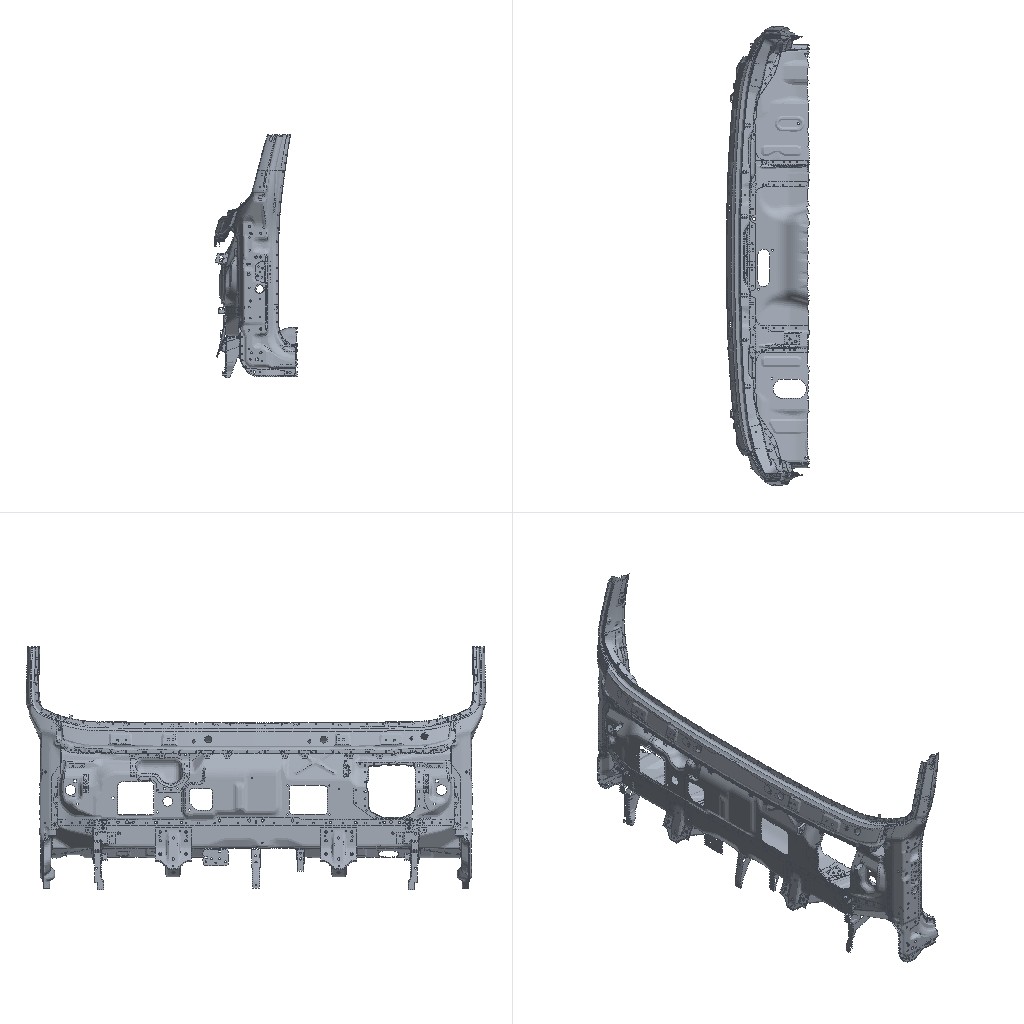Simulation study | nastran
Set-up summary:
category,name,step,type,value,unit,region
solver,nx_nastran
units,not stated in the deck,,not stated
analysis,deck,,static,static
analysis,solution,,SOL,101
load_step,SUBCASE 2,2,SUBCASE,SPC=11 LOAD=2
load_step,SUBCASE 3,3,SUBCASE,SPC=11 LOAD=3
load_step,SUBCASE 4,4,SUBCASE,SPC=11 LOAD=4
load_step,SUBCASE 5,5,SUBCASE,SPC=11 LOAD=5
load_step,SUBCASE 6,6,SUBCASE,SPC=11 LOAD=6
load_step,SUBCASE 7,7,SUBCASE,SPC=11 LOAD=7
load_step,SUBCASE 8,8,SUBCASE,SPC=11 LOAD=8
load_step,SUBCASE 9,9,SUBCASE,SPC=11 LOAD=9
load_step,SUBCASE 10,10,SUBCASE,SPC=11 LOAD=10
load_step,requested,,,9
mesh,nodes,,,77720
mesh,elements,,,69950
element_type,CHEXA,,unverified,613
element_type,CONM2,,mass,1
element_type,CQUAD4,,shell,64961
element_type,CTRIA3,,shell,4988
load,load commands in deck,,count,9
bc,support commands in deck,,count,1019
check,setup vs results,,match,"every grid point's frame and coordinates and every element id; grid points of CHEXA, CQUAD4, CTRIA3 elements"
Nastran input file, long lists of numbers shortened:
$$------------------------------------------------------------------------------$
$$                                                                              $
$$ NASTRAN Input Deck Generated by HyperMesh Version  : 9.0b121                 $
$$ Generated using HyperMesh-Nastran Template Version : 9.0b121
$$                                                                              $
$$   Template:  general                                                         $
$$                                                                              $
$$------------------------------------------------------------------------------$
$$------------------------------------------------------------------------------$
$$                      Executive Control Cards                                 $
$$------------------------------------------------------------------------------$
SOL 101
CEND
$$------------------------------------------------------------------------------$
$$                      Case Control Cards                                      $
$$------------------------------------------------------------------------------$
  DISPLACEMENT = ALL
$
$HMNAME LOADSTEP               2"Rx"
SUBCASE       2
  LABEL=   Rx
  SPC =       11
  LOAD =        2
$
$HMNAME LOADSTEP               3"Ry"
SUBCASE       3
  LABEL=   Ry
  SPC =       11
  LOAD =        3
$
$HMNAME LOADSTEP               4"Rz"
SUBCASE       4
  LABEL=   Rz
  SPC =       11
  LOAD =        4
$
$HMNAME LOADSTEP               5"Mx"
SUBCASE       5
  LABEL=   Mx
  SPC =       11
  LOAD =        5
$
$HMNAME LOADSTEP               6"My"
SUBCASE       6
  LABEL=   My
  SPC =       11
  LOAD =        6
$
$HMNAME LOADSTEP               7"Mz"
SUBCASE       7
  LABEL=   Mz
  SPC =       11
  LOAD =        7
$
$HMNAME LOADSTEP               8"Lx"
SUBCASE       8
  LABEL=   Lx
  SPC =       11
  LOAD =        8
$
$HMNAME LOADSTEP               9"Ly"
SUBCASE       9
  LABEL=   Ly
  SPC =       11
  LOAD =        9
$
$HMNAME LOADSTEP              10"Lz"
SUBCASE      10
  LABEL=   Lz
  SPC =       11
  LOAD =       10
$$------------------------------------------------------------------------------$
$$                      Bulk Data Cards                                         $
$$------------------------------------------------------------------------------$
BEGIN BULK
PARAM,POST,-1
$$
$$  GRID Data
$$
GRID         150        -903.017-1033.041012.706
GRID         536        -985.883-1013.11735.4542
$ (77718 more lines like these left out)
$$
$$  SPOINT Data
$$
$
$  CONM2 Elements
$
CONM2    103453984121617       00.00412 0.0     0.0     0.0
$
$HMMOVE 84022690
$        1034539
$
$$
$$------------------------------------------------------------------------------$
$$             Group Definitions                                                $
$$------------------------------------------------------------------------------$
$
$ RBE2 Elements - Single dependent node
$
RBE2      346590 3663307  123456 3657894
RBE2      346592 3663309  123456 3657892
$ (23 more lines like these left out)
$
$HMMOVE 57005014
$         346590  346592THRU      346597  346600THRU      346603  346605THRU
$         346608  346610THRU      346612  346614THRU      346620
$
$$
$$ RBE2 Elements - Multiple dependent nodes
$$
RBE2      346588 3663313  123456 3658184 3658185
RBE2      346589 3663312  123456 3657889 3658186
$ (98 more lines like these left out)
$
$HMMOVE 57005014
$         346588THRU      346589  346591  346598THRU      346599  346604  346609
$         346613  346621  346623THRU      346634 1034541THRU     1034542 1034540
$
$
$  RBE3 Elements
$
RBE3      326301         3755368  1234560.294793     123 37252000.075522+
+            123 37251970.128418     123 37251930.501266     123 3725196
RBE3      326302         3755369  1234560.049321     123 37252000.318302+
+            123 37251970.547536     123 37251930.084841     123 3725196
$ (9804 more lines like these left out)
$
$HMMOVE 57005012
$         326301THRU      326304  326306THRU      326313  326315THRU      326322
$         326324THRU      326331  326333THRU      326336  326427THRU      326430
$ (227 more lines like these left out)
CTRIA3    143987       2   55842   55843   55841
CTRIA3    144058       2   55842   55841   55996
$ (4986 more lines like these left out)
$
$HMMOVE       16
$         143987  144058  170026  170031  170036THRU      170037  170041  170048
$         170053  170057THRU      170058  189522  189524  198834THRU      198835
$ (604 more lines like these left out)
CQUAD4    170025       2   86431   86432   86426   86427
CQUAD4    170027       2   86442   86467   86451   86441
$ (64959 more lines like these left out)
$
$HMMOVE       16
$         170025  170027THRU      170030  170032THRU      170035  170038THRU
$         170040  170042THRU      170047  170049THRU      170052  170054THRU
$ (1536 more lines like these left out)
CHEXA     326305      10 3755368 3755369 3755370 3755371 3755372 3755373+
+        3755374 3755375
CHEXA     326314      10 3755377 3755380 3755379 3755378 3755381 3755384+
+        3755383 3755382
$ (1222 more lines like these left out)
$
$HMMOVE 57005011
$         326305  326314  326323  326332  326431  326440  326449  326458  326467
$         326476  326629  326638  326647  326656  326665  326674  326683  326692
$ (251 more lines like these left out)
PSHELL         1       10.8            1               1
$
$HMNAME PROP                   2"120" 4
$HWCOLOR PROP                  2       3
PSHELL         2       11.2            1               1
$
$HMNAME PROP                   3"180" 4
$HWCOLOR PROP                  3       3
PSHELL         3       11.8            1               1
$
$HMNAME PROP                   4"100" 4
$HWCOLOR PROP                  4       3
PSHELL         4       11.0            1               1
$
$HMNAME PROP                   5"150" 4
$HWCOLOR PROP                  5       3
PSHELL         5       11.5            1               1
$
$HMNAME PROP                   6"250" 4
$HWCOLOR PROP                  6       3
PSHELL         6       12.5            1               1
$
$HMNAME PROP                   7"200" 4
$HWCOLOR PROP                  7       3
PSHELL         7       12.0            1               1
$$
$$  PSOLID Data
$
$HMNAME PROP                  10"spot" 5
$HWCOLOR PROP                 10       3
PSOLID        10       1
$$
$$------------------------------------------------------------------------------$
$$                      Material Definition Cards                               $
$$------------------------------------------------------------------------------$
$$--------------------------------------------------------------
$$ HYPERMESH TAGS
$$--------------------------------------------------------------
$$BEGIN TAGS
$$END TAGS
$$
$$  MAT1 Data
$
$HMNAME MAT                    1"steel" "MAT1"
$HWCOLOR MAT                   1       3
MAT1           1210000.0        0.3     1.60E-08
$$
$$
$$
$$------------------------------------------------------------------------------$
$ (61 more lines like these left out)
SPC           11 3750681  1234560.0
SPC           11 3750682  1234560.0
SPC           11 3751236  1234560.0
SPC           11 3751237  1234560.0
$ (1015 more lines like these left out)
$$
$$  FORCE Data
$$
FORCE          284121625       01.0     100.0   0.0     0.0
FORCE          384121625       01.0     0.0     100.0   0.0
FORCE          484121625       01.0     0.0     0.0     100.0
FORCE          584121629       01.0     100.0   0.0     0.0
FORCE          684121629       01.0     0.0     100.0   0.0
FORCE          784121629       01.0     0.0     0.0     100.0
FORCE          884121633       01.0     100.0   0.0     0.0
FORCE          984121633       01.0     0.0     100.0   0.0
FORCE         1084121633       01.0     0.0     0.0     100.0
$HMASSEM 5400100       7 sidebody_L
$HMASSEM_IDS    540010105400303054003020540011105400112054003010
$HMASSEM 5400200       6 sidebody_R
$HMASSEM_IDS    540021105400212054004010540040205400403054002010
$HMASSEM      28       4 5300010
$HMASSEM_IDS          16      17      18      19      20      21      22      24
$HMASSEM_IDS          25      26
$HMASSEM       1       3 REAR_FLOOR
$HMASSEM_IDS    5100301051001110510052115100451051004210510048115100431151004610
$HMASSEM_IDS    5100411051002110510044105100601051009710510062115100471051004511
$HMASSEM_IDS    5100561351005410510064105100561051005611510056125100431051005311
$HMASSEM_IDS    510050105100341051009711
$
ENDDATA
Results summary:
result,analysis,,,static
result,last_loadstep,,,9
result,primary field,,,displacements
result,max displacement,,,0.7916,model units